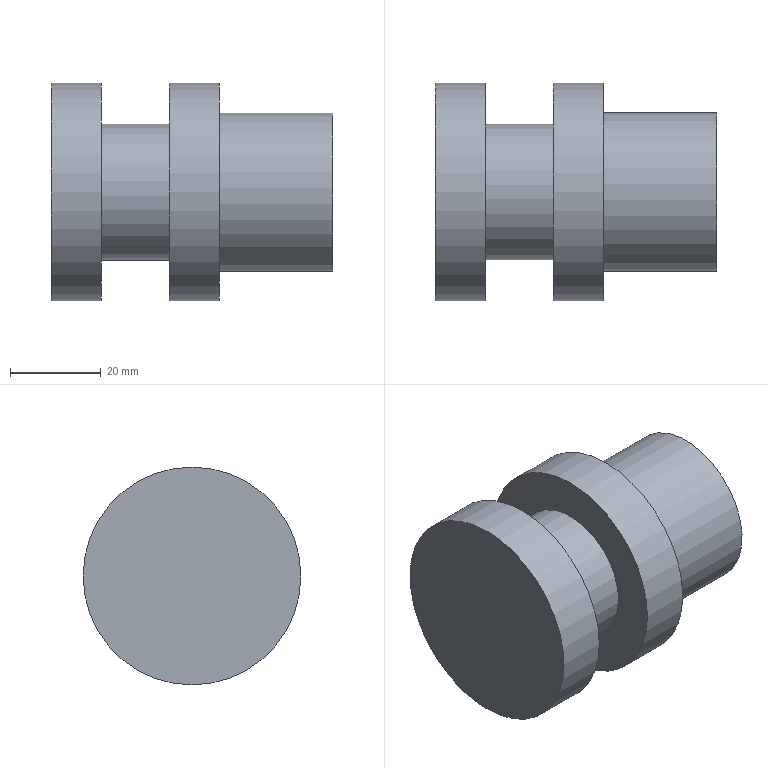Part | STEP file | Tube necking machine_id614_x_t | 1 solid | 15 faces | box 62 x 48 x 48 mm | volume 70559 mm3 | plane 6 | cylinder 6 | spline 2 | cone 1 | commonest cylinder face diameters 48 x2 21 x1 24 x1 30 x1 35 x1